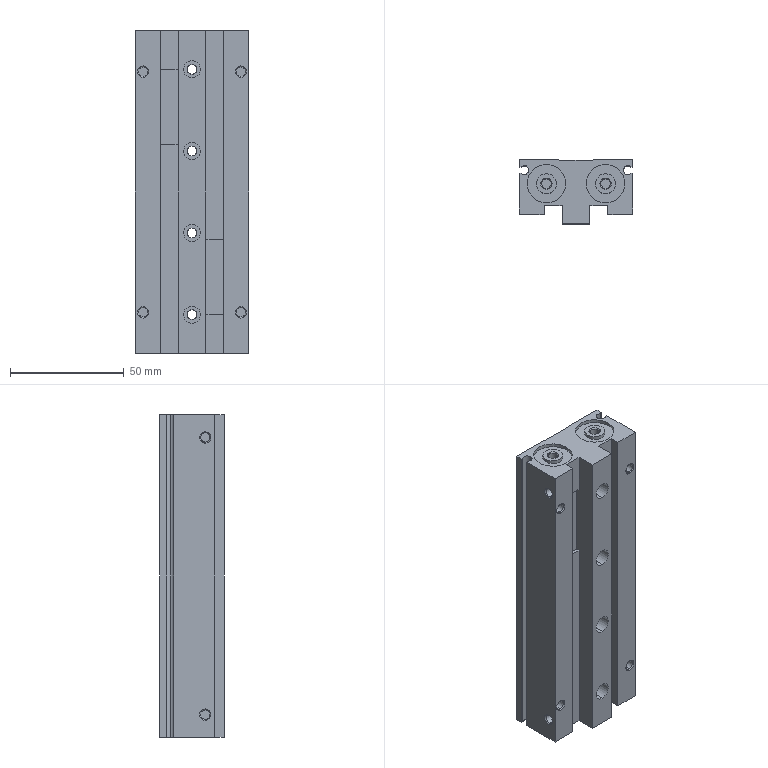Part | SolidWorks | features BaseBody 1 | 1 solid | 152 faces | box 50 x 28.3 x 142 mm | volume 158930 mm3 | cylinder 64 | plane 60 | cone 28 | commonest cylinder face diameters 4.134 x28 4 x8 4.3 x8 7.5 x8 17 x8 8.8 x4